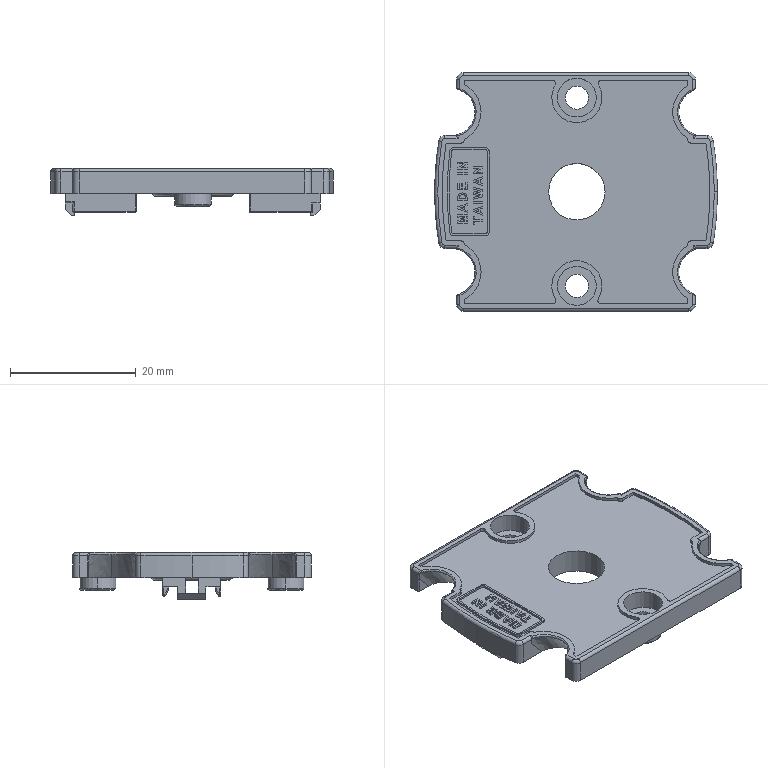Part | STEP file | PCS-02C2-3_1_2.stp | 1 solid | 540 faces | box 45.039 x 38 x 7.5 mm | volume 4082 mm3 | plane 277 | cylinder 176 | torus 41 | spline 32 | sphere 14 | commonest cylinder face diameters 0.4 x61 1 x48 2 x8 7.5 x6 8 x6 9.9 x6